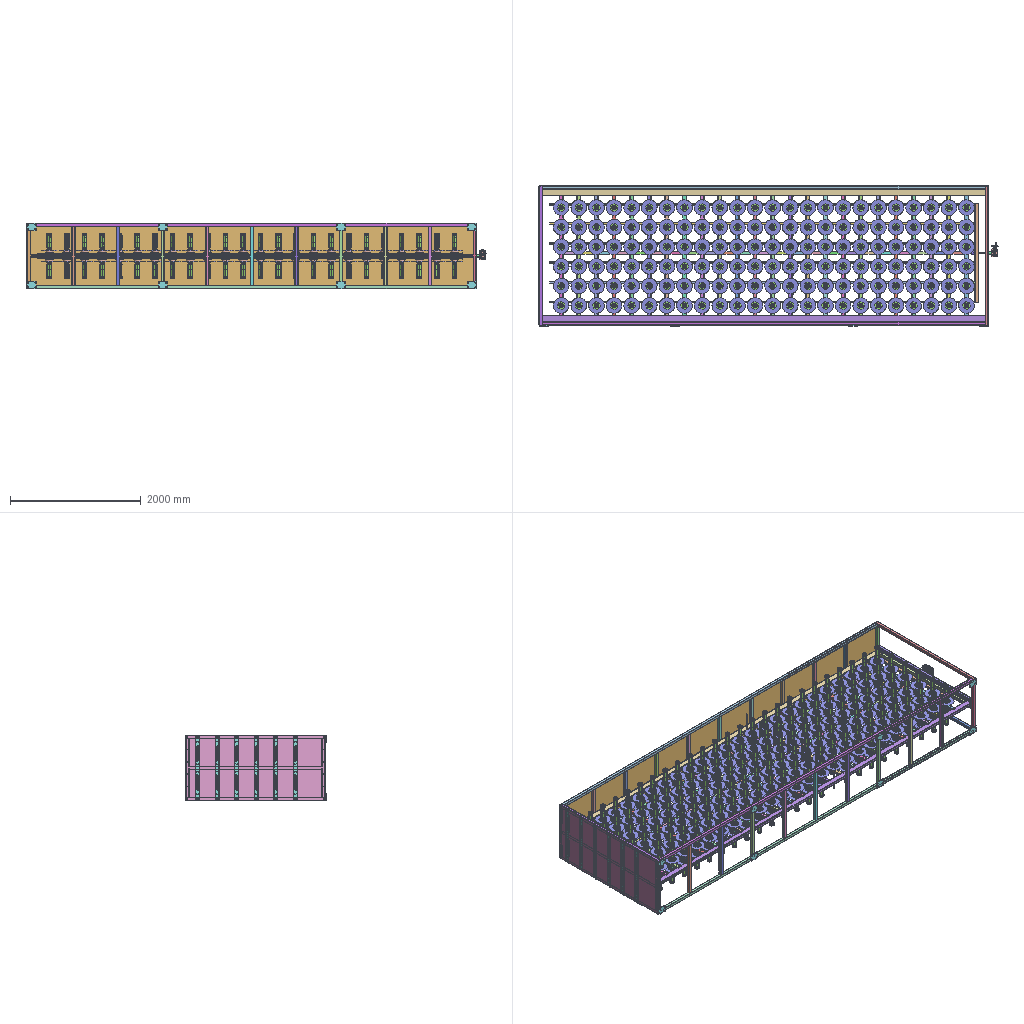Assembly | SolidWorks | 34 different items | 843 placed | box 7048 x 2145 x 1000 mm
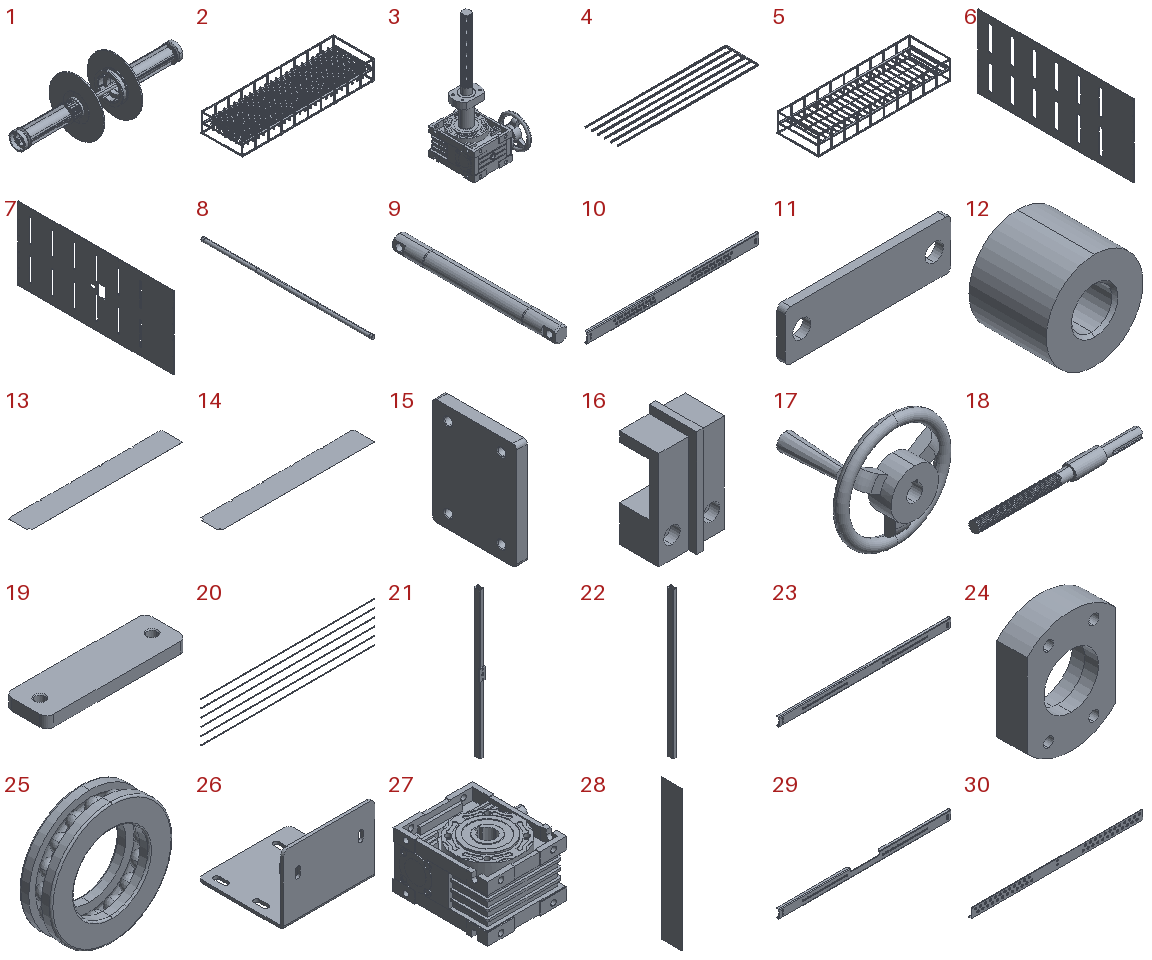Parts list (item | name | quantity | parent item | size | volume | features):
1 | (subassembly) | x144 | in 2 | 694.8 x 240 x 240 mm | 1341912 mm3 | features CompositeCurve 3
2 | (subassembly) | x1 | - | - | 274546419 mm3 | features ReferencePattern 238, LocalLPattern 4, MirrorCompFeat 2, LayoutProfileFeature 1
3 | (subassembly) | x1 | - | 219 x 160 x 404 mm | 1526813 mm3 | -
4 | (subassembly) | x1 | - | 6573 x 1530 x 100 mm | 13010460 mm3 | features ReferencePattern 111, LocalLPattern 3
5 | - | x1 | in 2 | - | 76543847 mm3 | features WeldCornerFeat 13, LPattern 7, HoleWzd 5, ICE 5, MoveCopyBody 4, WeldMemberFeat 4, 3DProfileFeature 1, Cut 1, MirrorSolid 1, WeldmentFeature 1
6 | - | x1 | - | 5 x 2120 x 990 mm | 9387989 mm3 | features LPattern 7, ICE 5, MirrorPattern 4, Fillet 2, HoleWzd 2, Extrusion 1
7 | - | x1 | - | 5 x 2120 x 990 mm | 9826354 mm3 | features LPattern 7, ICE 5, MirrorPattern 4, Fillet 2, HoleWzd 2, Extrusion 1
8 | - | x144 | in 1 | 15 x 688 x 15 mm | 121464 mm3 | features ICE 2, Chamfer 1, Extrusion 1, MirrorPattern 1
9 | - | x90 | in 4 | 12 x 130 x 12 mm | 13909 mm3 | features ICE 3, MirrorPattern 3, Chamfer 1, Extrusion 1
10 | - | x6 | - | 990 x 15 x 60 mm | 154443 mm3 | features ICE 3, LPattern 2, MirrorPattern 2, EdgeFlange 1, Fillet 1, FlatPattern 1, HoleWzd 1, SMBaseFlange 1, SheetMetal 1
11 | - | x12 | in 4 | 100 x 5 x 30 mm | 14011 mm3 | features Extrusion 1, Fillet 1, ICE 1
12 | - | x1 | in 4 | 50 x 40 x 50 mm | 64605 mm3 | features Extrusion 1, HoleWzd 1
13 | - | x1 | in 2 | 3434 x 480 x 1.2 mm | 1967250 mm3 | features Cut 2, Fillet 2, FlatPattern 1, ICE 1, SMBaseFlange 1, SheetMetal 1
14 | - | x1 | in 2 | 3434 x 480 x 1.2 mm | 1964220 mm3 | features Fillet 2, ICE 2, Cut 1, FlatPattern 1, SMBaseFlange 1, SheetMetal 1
15 | - | x8 | in 2 | 14 x 110 x 140 mm | 210665 mm3 | features Extrusion 1, Fillet 1, HoleWzd 1
16 | - | x96 | in 2 | 40 x 29 x 65 mm | 34575 mm3 | features ICE 5, Extrusion 1, HoleWzd 1
17 | - | x1 | in 3 | 100 x 75 x 100 mm | 59765 mm3 | features ICE 4, 3DProfileFeature 1, Fillet 1, Revolution 1, Sweep 1
18 | - | x1 | in 3 | 400 x 35 x 35 mm | 215314 mm3 | features ICE 3, Chamfer 1, Extrusion 1, HoleWzd 1, SweepThread 1
19 | - | x12 | in 4 | 100 x 30 x 8 mm | 23238 mm3 | features Extrusion 1, Fillet 1, HoleWzd 1
20 | - | x2 | in 4 | 6500 x 15 x 1530 mm | 5917812 mm3 | features 3DProfileFeature 1, Cut 1, LPattern 1, WeldMemberFeat 1, WeldmentFeature 1
21 | - | x1 | in 4 | 60 x 70 x 1530 mm | 886735 mm3 | features ICE 3, Fillet 1, WeldMemberFeat 1, WeldmentFeature 1
22 | - | x1 | in 4 | 40 x 60 x 1590 mm | 859909 mm3 | features Cut 1, WeldMemberFeat 1, WeldmentFeature 1
23 | - | x6 | - | 990 x 15 x 50 mm | 140813 mm3 | features ICE 2, EdgeFlange 1, Fillet 1, FlatPattern 1, HoleWzd 1, LPattern 1, MirrorPattern 1, SMBaseFlange 1, SheetMetal 1
24 | - | x1 | in 3 | 58 x 20 x 80 mm | 56726 mm3 | features ICE 3, Extrusion 1, HoleWzd 1
25 | - | x2 | in 3 | 42 x 11 x 42 mm | 6942 mm3 | features Revolution 3, CirPattern 1, Fillet 1
26 | - | x1 | - | 160 x 150 x 120 mm | 225790 mm3 | features ICE 3, EdgeFlange 1, Fillet 1, FlatPattern 1, Gusset 1, SMBaseFlange 1, SheetMetal 1
27 | - | x1 | in 3 | 164 x 144 x 92 mm | 1188126 mm3 | features ICE 59, CirPattern 14, Fillet 9, Revolution 9, Chamfer 7, MirrorPattern 3, DeleteBody 2, RevCut 2, Extrusion 1, MirrorSolid 1, SketchPattern 1
28 | - | x1 | - | 1.2 x 990 x 6870 mm | 8161457 mm3 | features Fillet 1, FlatPattern 1, SMBaseFlange 1, SheetMetal 1
29 | - | x1 | - | 990 x 15 x 50 mm | 130512 mm3 | features ICE 3, Fillet 2, EdgeFlange 1, FlatPattern 1, HoleWzd 1, LPattern 1, MirrorPattern 1, SMBaseFlange 1, SheetMetal 1
30 | - | x12 | - | 700 x 15 x 40 mm | 66578 mm3 | features ICE 3, LPattern 2, MirrorPattern 2, EdgeFlange 1, Fillet 1, FlatPattern 1, SMBaseFlange 1, SheetMetal 1
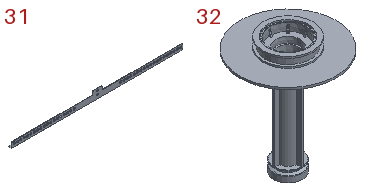31 | - | x1 | - | 720 x 15 x 40 mm | 44933 mm3 | features ICE 2, EdgeFlange 1, Fillet 1, FlatPattern 1, LPattern 1, MirrorPattern 1, SMBaseFlange 1, SheetMetal 1
32 | - | x288 | in 1 | 240 x 240 x 292.1 mm | 610223 mm3 | features MoveCopyBody 2, MBimport 1, MoveFace 1
33 | DNW aluminium alloy split clamp collar series[DNW-30×10-12] | x1 | - | - | - | -
34 | carbon fibre yarn roll | x1 | - | - | - | -
Mates (type | each side: item.copy, entity, surface, feature):
In the top assembly
Coincident | 5.1 face plane LPattern2 | 30.1 face plane Base-Flange1
Width | 5.1 face plane Gb/6728-1986 rectangular hollow section 060 X 40 X 3 | 5.1 face plane Gb/6728-1986 rectangular hollow section 060 X 40 X 3 | 20.1 face plane Gb/6728-1986 rectangular hollow section 030 X 20 X 2 | 20.2 face plane Gb/6728-1986 rectangular hollow section 030 X 20 X 2
Coincident | 16.1 face plane Boss-Extrude4 | 20.2 face plane Gb/6728-1986 rectangular hollow section 030 X 20 X 2
Width | 30.1 face plane Base-Flange1 | 30.1 face plane Base-Flange1 | 5.1 face plane LPattern2 | 5.1 face plane LPattern2
Coincident | 5.1 face plane LPattern2 | 31.1 face plane Base-Flange1
Concentric | 5.1 face cylinder LPattern7 | 31.1 face cylinder Cut-Extrude1 | 2 times
Concentric | 5.1 face cylinder Boss-Extrude4 | 18.1 face cylinder Boss-Extrude2
Coincident | 5.1 face plane Boss-Extrude4 | 24.1 face plane Boss-Extrude1
Coincident | 5.1 face plane Boss-Extrude3 | 26.1 face plane Base-Flange1
Slot | 26.1 face cylinder Cut-Extrude9 | 27.1 face cylinder Cut-Extrude5
Slot | 27.1 face cylinder Cut-Extrude5 | 26.1 face cylinder Cut-Extrude9
Parallel | 5.1 face plane Gb/t 6728-2002 square hollow section 050x30 | 27.1 face plane Boss-Extrude1
Coincident | 27.1 face plane Boss-Extrude1 | 26.1 face plane Edge-Flange1
Coincident | 5.1 face plane Gb/t 6728-2002 square hollow section 050x30 | 7.1 face plane Boss-Extrude1
Width | 5.1 face plane Gb/t 6728-2002 square hollow section 050x30 | 5.1 face plane Gb/t 6728-2002 square hollow section 050x30 | 7.1 face plane Boss-Extrude1 | 7.1 face plane Boss-Extrude1 | 2 times
Coincident | 7.1 face plane Boss-Extrude1 | 23.1 face plane Base-Flange1
Width | 5.1 face plane Gb/t 6728-2002 square hollow section 050x30 | 5.1 face plane Gb/t 6728-2002 square hollow section 050x30 | 23.1 face plane Base-Flange1 | 23.1 face plane Base-Flange1
DistanceDim | 23.1 face plane Edge-Flange1 | 7.1 face plane Boss-Extrude1
Coincident | 5.1 face plane Gb/t 6728-2002 square hollow section 050x30 | 6.1 face plane Boss-Extrude1
Width | 6.1 face plane Boss-Extrude1 | 6.1 face plane Boss-Extrude1 | 5.1 face plane Gb/t 6728-2002 square hollow section 050x30 | 5.1 face plane Gb/t 6728-2002 square hollow section 050x30 | 2 times
Coincident | 6.1 face plane Boss-Extrude1 | 10.1 face plane Base-Flange1
Width | 10.1 face plane Base-Flange1 | 10.1 face plane Base-Flange1 | 6.1 face plane Boss-Extrude1 | 6.1 face plane Boss-Extrude1
Slot | 10.1 face cylinder Cut-Extrude2 | 6.1 face cylinder M7 Clearance Hole2
Coincident | 23.2 face plane Base-Flange1 | 29.1 face plane Base-Flange1
Coincident | 7.1 face plane Boss-Extrude1 | 29.1 face plane Base-Flange1
Slot | 29.1 face cylinder Cut-Extrude2 | 7.1 face cylinder LPattern7
Coincident | 5.1 face plane Gb/t 6728-2002 square hollow section 050x30 | 28.1 face plane Base-Flange1
Width | 28.1 face plane Base-Flange1 | 28.1 face plane Base-Flange1 | 5.1 face plane Gb/t 6728-2002 square hollow section 050x30 | 5.1 face plane Gb/t 6728-2002 square hollow section 050x30
Width | 5.1 face plane Gb/t 6728-2002 square hollow section 050x30 | 5.1 face plane Gb/t 6728-2002 square hollow section 050x30 | 28.1 face plane Base-Flange1 | 28.1 face plane Base-Flange1
Coincident | 5.1 face plane LPattern2 | 30.2 face plane Base-Flange1
Concentric | 5.1 face cylinder LPattern7 | 30.2 face cylinder Cut-Extrude1
Coincident | 5.1 face plane LPattern2 | 16.2 face plane Boss-Extrude1
Concentric | 5.1 face cylinder LPattern6 | 16.2 face cylinder CBORE for M5 Hexagon socket head cap screws1 | 2 times
In subassembly 4
Coincident | 20.3 face plane Gb/6728-1986 rectangular hollow section 030 X 20 X 2 | 20.4 face plane Gb/6728-1986 rectangular hollow section 030 X 20 X 2 | 2 times
DistanceDim | 20.3 face plane Gb/6728-1986 rectangular hollow section 030 X 20 X 2 | 20.4 face plane Gb/6728-1986 rectangular hollow section 030 X 20 X 2
Coincident | 20.3 face plane Gb/6728-1986 rectangular hollow section 030 X 20 X 2 | 11.1 face plane Boss-Extrude1
Width | 11.2 face plane Boss-Extrude1 | 11.2 face plane Boss-Extrude1 | 22.1 face plane Gb/6728-1986 rectangular hollow section 060 X 40 X 3 | 22.1 face plane Gb/6728-1986 rectangular hollow section 060 X 40 X 3
Coincident | 11.2 face plane Boss-Extrude1 | 22.1 face plane Gb/6728-1986 rectangular hollow section 060 X 40 X 3
Coincident | 11.3 face plane Boss-Extrude1 | 22.1 face plane Gb/6728-1986 rectangular hollow section 060 X 40 X 3
Width | 20.3 face plane Gb/6728-1986 rectangular hollow section 030 X 20 X 2 | 20.4 face plane Gb/6728-1986 rectangular hollow section 030 X 20 X 2 | 21.1 face plane Gb/6728-1986 rectangular hollow section 060 X 40 X 3 | 21.1 face plane Gb/6728-1986 rectangular hollow section 060 X 40 X 3
Coincident | 11.4 face plane Boss-Extrude1 | 21.1 face plane Gb/6728-1986 rectangular hollow section 060 X 40 X 3
Coincident | 11.1 face plane Boss-Extrude1 | 21.1 face plane Gb/6728-1986 rectangular hollow section 060 X 40 X 3
Concentric | 21.1 face cylinder Boss-Extrude1 | 12.1 face cylinder Boss-Extrude1
Coincident | 21.1 face plane Boss-Extrude1 | 12.1 face plane Boss-Extrude1
Concentric | 20.4 face cylinder Cut-Extrude1 | 9.1 face cylinder Boss-Extrude1
Width | 9.1 face plane Boss-Extrude1 | 9.1 face plane Boss-Extrude1 | 20.3 face plane Gb/6728-1986 rectangular hollow section 030 X 20 X 2 | 20.4 face plane Gb/6728-1986 rectangular hollow section 030 X 20 X 2
Coincident | 20.3 face plane Gb/6728-1986 rectangular hollow section 030 X 20 X 2 | 19.1 face plane Boss-Extrude1 | 2 times
Width | 20.3 face plane Gb/6728-1986 rectangular hollow section 030 X 20 X 2 | 20.4 face plane Gb/6728-1986 rectangular hollow section 030 X 20 X 2 | 19.1 face plane Boss-Extrude1 | 19.1 face plane Boss-Extrude1
Concentric | 11.1 face cylinder Cut-Extrude1 | 19.1 face cylinder M8 Tapped Hole1
Coincident | 11.1 face plane Boss-Extrude1 | 19.1 face plane Boss-Extrude1
In subassembly 2
Concentric | 5.2 face cylinder Cut-Extrude2 | 8.1 face cylinder Boss-Extrude1
Width | 5.2 face plane Gb/6728-1986 rectangular hollow section 060 X 40 X 3 | 5.2 face plane Gb/6728-1986 rectangular hollow section 060 X 40 X 3 | 32.1 face plane bearing sleeve-1122.stp<1> | 32.2 face plane bearing sleeve-1122.stp<1>
Concentric | 5.2 face cylinder M5 Tapped Hole1 | 16.3 face cylinder CBORE for M5 Hexagon socket head cap screws1 | 2 times
Coincident | 5.2 face plane Gb/6728-1986 rectangular hollow section 060 X 40 X 3 | 16.3 face plane Boss-Extrude1
Coincident | 5.2 face plane Mirror1 | 14.1 face plane Base-Flange1
Coincident | 5.2 edge | 14.1 face plane Base-Flange1 | 2 times
Coincident | 5.2 face plane Gb/t 6728-2002 square hollow section 050x30 | 13.1 face plane Base-Flange1
Coincident | 5.2 edge | 13.1 face plane Base-Flange1 | 2 times
Coincident | 5.2 face plane Gb/t 6728-2002 square hollow section 050x30 | 15.1 face plane Boss-Extrude1 | 3 times
Coincident | 5.2 face plane Gb/t 6728-2002 square hollow section 050x30 | 15.2 face plane Boss-Extrude1 | 3 times
In subassembly 1
Concentric | 8.2 face cylinder Boss-Extrude1 | 32.3 face cone bearing sleeve-1122.stp<1>
Coincident | 8.2 edge | 32.3 face plane bearing sleeve-1122.stp<1>
Concentric | 8.2 face cylinder Boss-Extrude1 | 32.4 face cone bearing sleeve-1122.stp<1>
Coincident | 8.2 edge | 32.4 face plane bearing sleeve-1122.stp<1>
In subassembly 3
Coincident | 17.1 face plane Boss-Extrude1 | 27.2 face plane Revolve3
Concentric | 17.1 face cylinder Cut-Extrude3 | 27.2 face cylinder Revolve3
Concentric | 18.2 face cylinder Cut-Extrude2 | 27.2 face cylinder Cut-Revolve1
Coincident | 18.2 face plane Boss-Extrude1 | 27.2 face plane Boss-Extrude5
Concentric | 18.2 face cylinder Cut-Extrude2 | 25.1 face cylinder Boss-Revolve3
Concentric | 18.2 face cylinder Cut-Extrude2 | 25.2 face cylinder Boss-Revolve3
Coincident | 18.2 face plane Boss-Extrude2 | 25.2 face plane Boss-Revolve3
Concentric | 18.2 face cylinder Boss-Extrude2 | 24.2 face cylinder Cut-Extrude1
Parallel | 27.2 face plane Boss-Extrude1 | 24.2 face plane Cut-Extrude3
Coincident | 25.2 face plane Base-Revolve | 24.2 face plane Boss-Extrude1